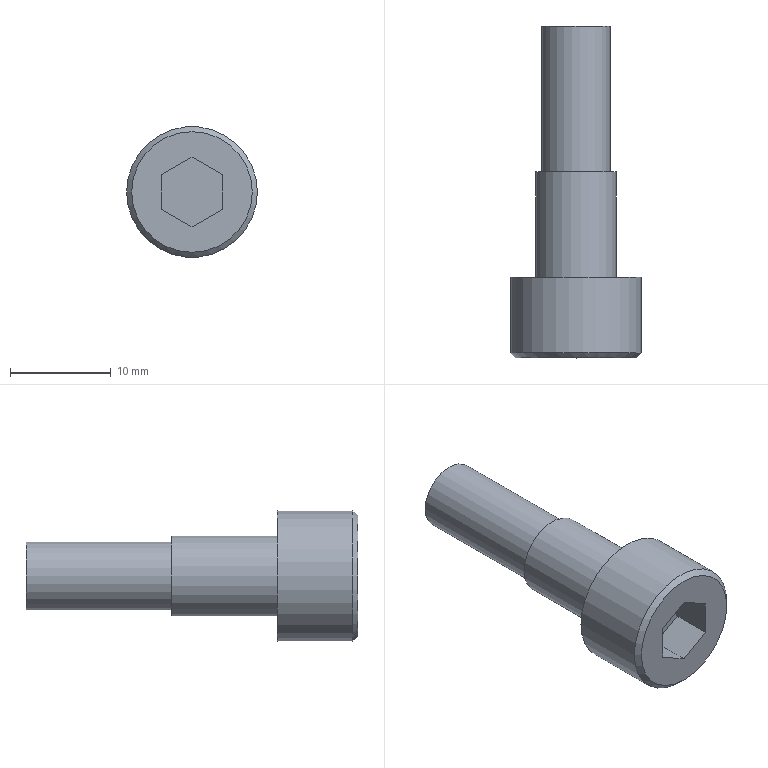Part | STEP file | M3-10_id1422_x_t | 1 solid | 15 faces | box 13 x 33 x 13 mm | volume 1987 mm3 | plane 11 | cylinder 3 | cone 1 | commonest cylinder face diameters 6.8 x1 8 x1 13 x1
STEP:
#1=CARTESIAN_POINT('',(-339.1,-292.5,-14.6));
#2=VERTEX_POINT('',#1);
#3=CARTESIAN_POINT('',(-342.5,-292.5,-14.6));
#4=DIRECTION('',(0.,1.,0.));
#5=DIRECTION('',(1.,0.,0.));
#6=AXIS2_PLACEMENT_3D('',#3,#4,#5);
#7=CIRCLE('',#6,3.4);
#8=EDGE_CURVE('',#2,#2,#7,.T.);
#9=ORIENTED_EDGE('',*,*,#8,.F.);
#10=EDGE_LOOP('',(#9));
#11=FACE_BOUND('',#10,.T.);
#12=CARTESIAN_POINT('',(-346.5,-292.5,-14.6));
#13=VERTEX_POINT('',#12);
#14=CARTESIAN_POINT('',(-342.5,-292.5,-14.6));
#15=DIRECTION('',(0.,-1.,0.));
#16=DIRECTION('',(-1.,0.,0.));
#17=AXIS2_PLACEMENT_3D('',#14,#15,#16);
#18=CIRCLE('',#17,4.);
#19=EDGE_CURVE('',#13,#13,#18,.T.);
#20=ORIENTED_EDGE('',*,*,#19,.F.);
#21=EDGE_LOOP('',(#20));
#22=FACE_BOUND('',#21,.T.);
#23=CARTESIAN_POINT('',(-342.5,-292.5,-14.6));
#24=DIRECTION('',(0.,1.,0.));
#25=DIRECTION('',(1.,0.,0.));
#26=AXIS2_PLACEMENT_3D('',#23,#24,#25);
#27=PLANE('',#26);
#28=ADVANCED_FACE('',(#11,#22),#27,.T.);
#29=CARTESIAN_POINT('',(-338.5,-303.,-14.6));
#30=VERTEX_POINT('',#29);
#31=CARTESIAN_POINT('',(-342.5,-303.,-14.6));
#32=DIRECTION('',(0.,-1.,0.));
#33=DIRECTION('',(1.,0.,0.));
#34=AXIS2_PLACEMENT_3D('',#31,#32,#33);
#35=CIRCLE('',#34,4.);
#36=EDGE_CURVE('',#30,#30,#35,.T.);
#37=ORIENTED_EDGE('',*,*,#36,.F.);
#38=EDGE_LOOP('',(#37));
#39=FACE_BOUND('',#38,.T.);
#40=ORIENTED_EDGE('',*,*,#19,.T.);
#41=EDGE_LOOP('',(#40));
#42=FACE_BOUND('',#41,.T.);
#43=CARTESIAN_POINT('',(-342.5,-292.5,-14.6));
#44=DIRECTION('',(0.,-1.,0.));
#45=DIRECTION('',(-1.,0.,0.));
#46=AXIS2_PLACEMENT_3D('',#43,#44,#45);
#47=CYLINDRICAL_SURFACE('',#46,4.);
#48=ADVANCED_FACE('',(#39,#42),#47,.T.);
#49=CARTESIAN_POINT('',(-345.9,-278.,-14.6));
#50=VERTEX_POINT('',#49);
#51=CARTESIAN_POINT('',(-342.5,-278.,-14.6));
#52=DIRECTION('',(0.,-1.,0.));
#53=DIRECTION('',(-1.,0.,0.));
#54=AXIS2_PLACEMENT_3D('',#51,#52,#53);
#55=CIRCLE('',#54,3.4);
#56=EDGE_CURVE('',#50,#50,#55,.T.);
#57=ORIENTED_EDGE('',*,*,#56,.F.);
#58=EDGE_LOOP('',(#57));
#59=FACE_OUTER_BOUND('',#58,.T.);
#60=CARTESIAN_POINT('',(-342.5,-278.,-14.6));
#61=DIRECTION('',(0.,1.,0.));
#62=DIRECTION('',(1.,0.,0.));
#63=AXIS2_PLACEMENT_3D('',#60,#61,#62);
#64=PLANE('',#63);
#65=ADVANCED_FACE('',(#59),#64,.T.);
#66=ORIENTED_EDGE('',*,*,#56,.T.);
#67=EDGE_LOOP('',(#66));
#68=FACE_BOUND('',#67,.T.);
#69=ORIENTED_EDGE('',*,*,#8,.T.);
#70=EDGE_LOOP('',(#69));
#71=FACE_BOUND('',#70,.T.);
#72=CARTESIAN_POINT('',(-342.5,-292.5,-14.6));
#73=DIRECTION('',(0.,1.,0.));
#74=DIRECTION('',(-1.,0.,0.));
#75=AXIS2_PLACEMENT_3D('',#72,#73,#74);
#76=CYLINDRICAL_SURFACE('',#75,3.4);
#77=ADVANCED_FACE('',(#68,#71),#76,.T.);
#78=CARTESIAN_POINT('',(-339.5,-311.,-16.332));
#79=VERTEX_POINT('',#78);
#80=CARTESIAN_POINT('',(-339.5,-311.,-12.868));
#81=VERTEX_POINT('',#80);
#82=CARTESIAN_POINT('',(-339.5,-311.,-16.332));
#83=DIRECTION('',(0.,0.,1.));
#84=VECTOR('',#83,1.);
#85=LINE('',#82,#84);
#86=EDGE_CURVE('',#79,#81,#85,.T.);
#87=ORIENTED_EDGE('',*,*,#86,.F.);
#88=CARTESIAN_POINT('',(-342.5,-311.,-18.064));
#89=VERTEX_POINT('',#88);
#90=CARTESIAN_POINT('',(-342.5,-311.,-18.064));
#91=DIRECTION('',(0.866,0.,0.5));
#92=VECTOR('',#91,1.);
#93=LINE('',#90,#92);
#94=EDGE_CURVE('',#89,#79,#93,.T.);
#95=ORIENTED_EDGE('',*,*,#94,.F.);
#96=CARTESIAN_POINT('',(-345.5,-311.,-16.332));
#97=VERTEX_POINT('',#96);
#98=CARTESIAN_POINT('',(-345.5,-311.,-16.332));
#99=DIRECTION('',(0.866,0.,-0.5));
#100=VECTOR('',#99,1.);
#101=LINE('',#98,#100);
#102=EDGE_CURVE('',#97,#89,#101,.T.);
#103=ORIENTED_EDGE('',*,*,#102,.F.);
#104=CARTESIAN_POINT('',(-345.5,-311.,-12.868));
#105=VERTEX_POINT('',#104);
#106=CARTESIAN_POINT('',(-345.5,-311.,-12.868));
#107=DIRECTION('',(0.,0.,-1.));
#108=VECTOR('',#107,1.);
#109=LINE('',#106,#108);
#110=EDGE_CURVE('',#105,#97,#109,.T.);
#111=ORIENTED_EDGE('',*,*,#110,.F.);
#112=CARTESIAN_POINT('',(-342.5,-311.,-11.136));
#113=VERTEX_POINT('',#112);
#114=CARTESIAN_POINT('',(-342.5,-311.,-11.136));
#115=DIRECTION('',(-0.866,0.,-0.5));
#116=VECTOR('',#115,1.);
#117=LINE('',#114,#116);
#118=EDGE_CURVE('',#113,#105,#117,.T.);
#119=ORIENTED_EDGE('',*,*,#118,.F.);
#120=CARTESIAN_POINT('',(-339.5,-311.,-12.868));
#121=DIRECTION('',(-0.866,0.,0.5));
#122=VECTOR('',#121,1.);
#123=LINE('',#120,#122);
#124=EDGE_CURVE('',#81,#113,#123,.T.);
#125=ORIENTED_EDGE('',*,*,#124,.F.);
#126=EDGE_LOOP('',(#87,#95,#103,#111,#119,#125));
#127=FACE_BOUND('',#126,.T.);
#128=CARTESIAN_POINT('',(-348.5,-311.,-14.6));
#129=VERTEX_POINT('',#128);
#130=CARTESIAN_POINT('',(-342.5,-311.,-14.6));
#131=DIRECTION('',(0.,-1.,0.));
#132=DIRECTION('',(-1.,0.,0.));
#133=AXIS2_PLACEMENT_3D('',#130,#131,#132);
#134=CIRCLE('',#133,6.);
#135=EDGE_CURVE('',#129,#129,#134,.T.);
#136=ORIENTED_EDGE('',*,*,#135,.T.);
#137=EDGE_LOOP('',(#136));
#138=FACE_BOUND('',#137,.T.);
#139=CARTESIAN_POINT('',(-342.5,-311.,-14.6));
#140=DIRECTION('',(0.,-1.,0.));
#141=DIRECTION('',(-1.,0.,0.));
#142=AXIS2_PLACEMENT_3D('',#139,#140,#141);
#143=PLANE('',#142);
#144=ADVANCED_FACE('',(#127,#138),#143,.T.);
#145=ORIENTED_EDGE('',*,*,#36,.T.);
#146=EDGE_LOOP('',(#145));
#147=FACE_BOUND('',#146,.T.);
#148=CARTESIAN_POINT('',(-349.,-303.,-14.6));
#149=VERTEX_POINT('',#148);
#150=CARTESIAN_POINT('',(-342.5,-303.,-14.6));
#151=DIRECTION('',(0.,-1.,0.));
#152=DIRECTION('',(-1.,0.,0.));
#153=AXIS2_PLACEMENT_3D('',#150,#151,#152);
#154=CIRCLE('',#153,6.5);
#155=EDGE_CURVE('',#149,#149,#154,.T.);
#156=ORIENTED_EDGE('',*,*,#155,.F.);
#157=EDGE_LOOP('',(#156));
#158=FACE_BOUND('',#157,.T.);
#159=CARTESIAN_POINT('',(-342.5,-303.,-14.6));
#160=DIRECTION('',(0.,1.,0.));
#161=DIRECTION('',(1.,0.,0.));
#162=AXIS2_PLACEMENT_3D('',#159,#160,#161);
#163=PLANE('',#162);
#164=ADVANCED_FACE('',(#147,#158),#163,.T.);
#165=CARTESIAN_POINT('',(-349.,-310.5,-14.6));
#166=VERTEX_POINT('',#165);
#167=CARTESIAN_POINT('',(-342.5,-310.5,-14.6));
#168=DIRECTION('',(0.,1.,0.));
#169=DIRECTION('',(-1.,0.,0.));
#170=AXIS2_PLACEMENT_3D('',#167,#168,#169);
#171=CIRCLE('',#170,6.5);
#172=EDGE_CURVE('',#166,#166,#171,.T.);
#173=ORIENTED_EDGE('',*,*,#172,.T.);
#174=EDGE_LOOP('',(#173));
#175=FACE_BOUND('',#174,.T.);
#176=ORIENTED_EDGE('',*,*,#155,.T.);
#177=EDGE_LOOP('',(#176));
#178=FACE_BOUND('',#177,.T.);
#179=CARTESIAN_POINT('',(-342.5,-303.,-14.6));
#180=DIRECTION('',(0.,-1.,0.));
#181=DIRECTION('',(-1.,0.,0.));
#182=AXIS2_PLACEMENT_3D('',#179,#180,#181);
#183=CYLINDRICAL_SURFACE('',#182,6.5);
#184=ADVANCED_FACE('',(#175,#178),#183,.T.);
#185=ORIENTED_EDGE('',*,*,#135,.F.);
#186=EDGE_LOOP('',(#185));
#187=FACE_BOUND('',#186,.T.);
#188=ORIENTED_EDGE('',*,*,#172,.F.);
#189=EDGE_LOOP('',(#188));
#190=FACE_BOUND('',#189,.T.);
#191=CARTESIAN_POINT('',(-342.5,-310.5,-14.6));
#192=DIRECTION('',(0.,1.,0.));
#193=DIRECTION('',(1.,0.,0.));
#194=AXIS2_PLACEMENT_3D('',#191,#192,#193);
#195=CONICAL_SURFACE('',#194,6.5,45.);
#196=ADVANCED_FACE('',(#187,#190),#195,.T.);
#197=ORIENTED_EDGE('',*,*,#86,.T.);
#198=CARTESIAN_POINT('',(-339.5,-307.,-12.868));
#199=VERTEX_POINT('',#198);
#200=CARTESIAN_POINT('',(-339.5,-307.,-12.868));
#201=DIRECTION('',(0.,1.,0.));
#202=VECTOR('',#201,1.);
#203=LINE('',#200,#202);
#204=EDGE_CURVE('',#81,#199,#203,.T.);
#205=ORIENTED_EDGE('',*,*,#204,.T.);
#206=CARTESIAN_POINT('',(-339.5,-307.,-16.332));
#207=VERTEX_POINT('',#206);
#208=CARTESIAN_POINT('',(-339.5,-307.,-16.332));
#209=DIRECTION('',(0.,0.,-1.));
#210=VECTOR('',#209,1.);
#211=LINE('',#208,#210);
#212=EDGE_CURVE('',#199,#207,#211,.T.);
#213=ORIENTED_EDGE('',*,*,#212,.T.);
#214=CARTESIAN_POINT('',(-339.5,-307.,-16.332));
#215=DIRECTION('',(0.,1.,0.));
#216=VECTOR('',#215,1.);
#217=LINE('',#214,#216);
#218=EDGE_CURVE('',#79,#207,#217,.T.);
#219=ORIENTED_EDGE('',*,*,#218,.F.);
#220=EDGE_LOOP('',(#197,#205,#213,#219));
#221=FACE_OUTER_BOUND('',#220,.T.);
#222=CARTESIAN_POINT('',(-339.5,-307.,-16.332));
#223=DIRECTION('',(1.,0.,0.));
#224=DIRECTION('',(0.,0.,1.));
#225=AXIS2_PLACEMENT_3D('',#222,#223,#224);
#226=PLANE('',#225);
#227=ADVANCED_FACE('',(#221),#226,.F.);
#228=ORIENTED_EDGE('',*,*,#124,.T.);
#229=CARTESIAN_POINT('',(-342.5,-307.,-11.136));
#230=VERTEX_POINT('',#229);
#231=CARTESIAN_POINT('',(-342.5,-307.,-11.136));
#232=DIRECTION('',(0.,1.,0.));
#233=VECTOR('',#232,1.);
#234=LINE('',#231,#233);
#235=EDGE_CURVE('',#113,#230,#234,.T.);
#236=ORIENTED_EDGE('',*,*,#235,.T.);
#237=CARTESIAN_POINT('',(-339.5,-307.,-12.868));
#238=DIRECTION('',(0.866,0.,-0.5));
#239=VECTOR('',#238,1.);
#240=LINE('',#237,#239);
#241=EDGE_CURVE('',#230,#199,#240,.T.);
#242=ORIENTED_EDGE('',*,*,#241,.T.);
#243=ORIENTED_EDGE('',*,*,#204,.F.);
#244=EDGE_LOOP('',(#228,#236,#242,#243));
#245=FACE_OUTER_BOUND('',#244,.T.);
#246=CARTESIAN_POINT('',(-339.5,-307.,-12.868));
#247=DIRECTION('',(0.5,0.,0.866));
#248=DIRECTION('',(-0.866,0.,0.5));
#249=AXIS2_PLACEMENT_3D('',#246,#247,#248);
#250=PLANE('',#249);
#251=ADVANCED_FACE('',(#245),#250,.F.);
#252=ORIENTED_EDGE('',*,*,#118,.T.);
#253=CARTESIAN_POINT('',(-345.5,-307.,-12.868));
#254=VERTEX_POINT('',#253);
#255=CARTESIAN_POINT('',(-345.5,-307.,-12.868));
#256=DIRECTION('',(0.,1.,0.));
#257=VECTOR('',#256,1.);
#258=LINE('',#255,#257);
#259=EDGE_CURVE('',#105,#254,#258,.T.);
#260=ORIENTED_EDGE('',*,*,#259,.T.);
#261=CARTESIAN_POINT('',(-342.5,-307.,-11.136));
#262=DIRECTION('',(0.866,0.,0.5));
#263=VECTOR('',#262,1.);
#264=LINE('',#261,#263);
#265=EDGE_CURVE('',#254,#230,#264,.T.);
#266=ORIENTED_EDGE('',*,*,#265,.T.);
#267=ORIENTED_EDGE('',*,*,#235,.F.);
#268=EDGE_LOOP('',(#252,#260,#266,#267));
#269=FACE_OUTER_BOUND('',#268,.T.);
#270=CARTESIAN_POINT('',(-342.5,-307.,-11.136));
#271=DIRECTION('',(-0.5,0.,0.866));
#272=DIRECTION('',(-0.866,0.,-0.5));
#273=AXIS2_PLACEMENT_3D('',#270,#271,#272);
#274=PLANE('',#273);
#275=ADVANCED_FACE('',(#269),#274,.F.);
#276=ORIENTED_EDGE('',*,*,#110,.T.);
#277=CARTESIAN_POINT('',(-345.5,-307.,-16.332));
#278=VERTEX_POINT('',#277);
#279=CARTESIAN_POINT('',(-345.5,-307.,-16.332));
#280=DIRECTION('',(0.,1.,0.));
#281=VECTOR('',#280,1.);
#282=LINE('',#279,#281);
#283=EDGE_CURVE('',#97,#278,#282,.T.);
#284=ORIENTED_EDGE('',*,*,#283,.T.);
#285=CARTESIAN_POINT('',(-345.5,-307.,-12.868));
#286=DIRECTION('',(0.,0.,1.));
#287=VECTOR('',#286,1.);
#288=LINE('',#285,#287);
#289=EDGE_CURVE('',#278,#254,#288,.T.);
#290=ORIENTED_EDGE('',*,*,#289,.T.);
#291=ORIENTED_EDGE('',*,*,#259,.F.);
#292=EDGE_LOOP('',(#276,#284,#290,#291));
#293=FACE_OUTER_BOUND('',#292,.T.);
#294=CARTESIAN_POINT('',(-345.5,-307.,-12.868));
#295=DIRECTION('',(-1.,0.,0.));
#296=DIRECTION('',(0.,0.,-1.));
#297=AXIS2_PLACEMENT_3D('',#294,#295,#296);
#298=PLANE('',#297);
#299=ADVANCED_FACE('',(#293),#298,.F.);
#300=ORIENTED_EDGE('',*,*,#102,.T.);
#301=CARTESIAN_POINT('',(-342.5,-307.,-18.064));
#302=VERTEX_POINT('',#301);
#303=CARTESIAN_POINT('',(-342.5,-307.,-18.064));
#304=DIRECTION('',(0.,1.,0.));
#305=VECTOR('',#304,1.);
#306=LINE('',#303,#305);
#307=EDGE_CURVE('',#89,#302,#306,.T.);
#308=ORIENTED_EDGE('',*,*,#307,.T.);
#309=CARTESIAN_POINT('',(-345.5,-307.,-16.332));
#310=DIRECTION('',(-0.866,0.,0.5));
#311=VECTOR('',#310,1.);
#312=LINE('',#309,#311);
#313=EDGE_CURVE('',#302,#278,#312,.T.);
#314=ORIENTED_EDGE('',*,*,#313,.T.);
#315=ORIENTED_EDGE('',*,*,#283,.F.);
#316=EDGE_LOOP('',(#300,#308,#314,#315));
#317=FACE_OUTER_BOUND('',#316,.T.);
#318=CARTESIAN_POINT('',(-345.5,-307.,-16.332));
#319=DIRECTION('',(-0.5,0.,-0.866));
#320=DIRECTION('',(0.866,0.,-0.5));
#321=AXIS2_PLACEMENT_3D('',#318,#319,#320);
#322=PLANE('',#321);
#323=ADVANCED_FACE('',(#317),#322,.F.);
#324=ORIENTED_EDGE('',*,*,#94,.T.);
#325=ORIENTED_EDGE('',*,*,#218,.T.);
#326=CARTESIAN_POINT('',(-342.5,-307.,-18.064));
#327=DIRECTION('',(-0.866,0.,-0.5));
#328=VECTOR('',#327,1.);
#329=LINE('',#326,#328);
#330=EDGE_CURVE('',#207,#302,#329,.T.);
#331=ORIENTED_EDGE('',*,*,#330,.T.);
#332=ORIENTED_EDGE('',*,*,#307,.F.);
#333=EDGE_LOOP('',(#324,#325,#331,#332));
#334=FACE_OUTER_BOUND('',#333,.T.);
#335=CARTESIAN_POINT('',(-342.5,-307.,-18.064));
#336=DIRECTION('',(0.5,0.,-0.866));
#337=DIRECTION('',(0.866,0.,0.5));
#338=AXIS2_PLACEMENT_3D('',#335,#336,#337);
#339=PLANE('',#338);
#340=ADVANCED_FACE('',(#334),#339,.F.);
#341=ORIENTED_EDGE('',*,*,#212,.F.);
#342=ORIENTED_EDGE('',*,*,#241,.F.);
#343=ORIENTED_EDGE('',*,*,#265,.F.);
#344=ORIENTED_EDGE('',*,*,#289,.F.);
#345=ORIENTED_EDGE('',*,*,#313,.F.);
#346=ORIENTED_EDGE('',*,*,#330,.F.);
#347=EDGE_LOOP('',(#341,#342,#343,#344,#345,#346));
#348=FACE_OUTER_BOUND('',#347,.T.);
#349=CARTESIAN_POINT('',(-342.5,-307.,-14.6));
#350=DIRECTION('',(0.,-1.,0.));
#351=DIRECTION('',(-1.,0.,0.));
#352=AXIS2_PLACEMENT_3D('',#349,#350,#351);
#353=PLANE('',#352);
#354=ADVANCED_FACE('',(#348),#353,.T.);
#355=CLOSED_SHELL('',(#28,#48,#65,#77,#144,#164,#184,#196,#227,#251,#275,#299,#323,#340,#354));
#356=MANIFOLD_SOLID_BREP('',#355);
#357=(LENGTH_UNIT()NAMED_UNIT(*)SI_UNIT(.MILLI.,.METRE.));
#358=UNCERTAINTY_MEASURE_WITH_UNIT(LENGTH_MEASURE(0.00002),#357,'','');
#359=(NAMED_UNIT(*)PLANE_ANGLE_UNIT()SI_UNIT($,.RADIAN.));
#360=PLANE_ANGLE_MEASURE_WITH_UNIT(PLANE_ANGLE_MEASURE(0.01745),#359);
#361=DIMENSIONAL_EXPONENTS(0.,0.,0.,0.,0.,0.,0.);
#362=(CONVERSION_BASED_UNIT('DEGREE',#360)NAMED_UNIT(#361)PLANE_ANGLE_UNIT());
#363=(NAMED_UNIT(*)SI_UNIT($,.STERADIAN.)SOLID_ANGLE_UNIT());
#364=(GEOMETRIC_REPRESENTATION_CONTEXT(3)GLOBAL_UNCERTAINTY_ASSIGNED_CONTEXT((#358))GLOBAL_UNIT_ASSIGNED_CONTEXT((#357,#362,#363))REPRESENTATION_CONTEXT('',''));
#365=ADVANCED_BREP_SHAPE_REPRESENTATION('',(#356),#364);